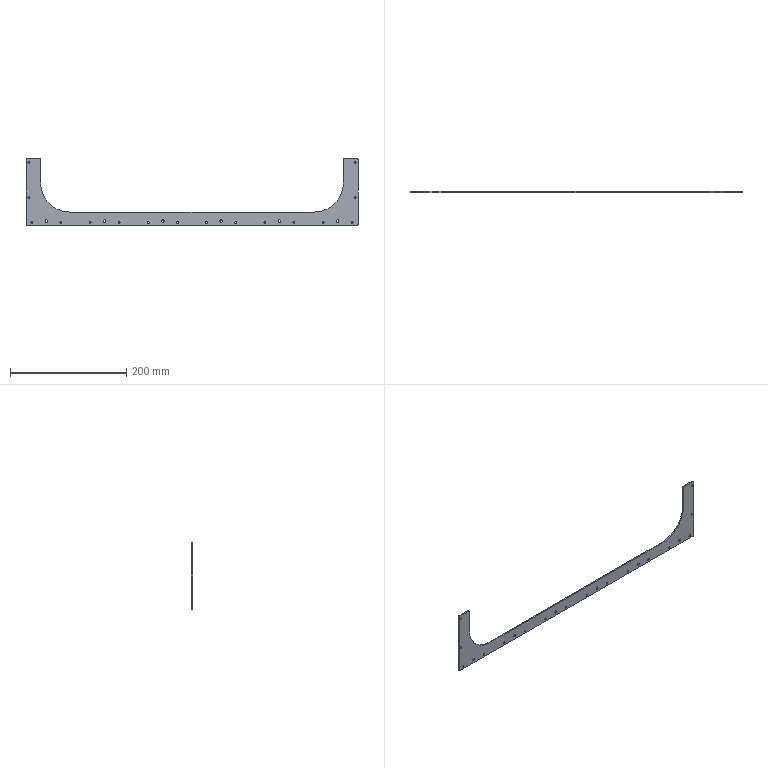Part | STEP file | 1 solid | 62 faces | box 570 x 2 x 115 mm | volume 37091 mm3 | cylinder 52 | plane 10 | commonest cylinder face diameters 3.3 x32 4.5 x12 4 x6 100 x2